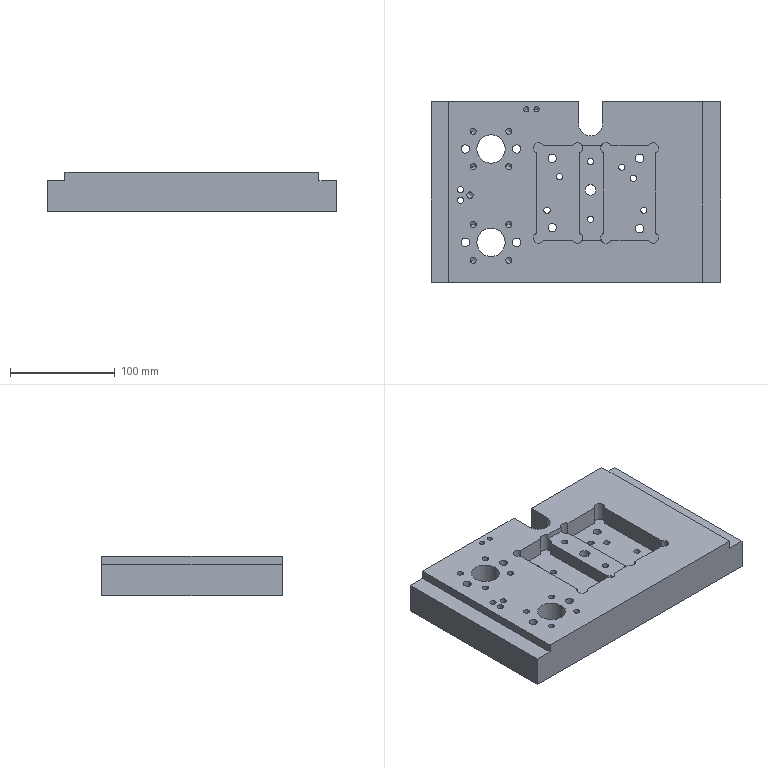Part | 1 solid | 119 faces | box 275.4 x 172 x 38 mm | volume 1497527 mm3 | cylinder 71 | plane 26 | cone 22 | commonest cylinder face diameters 6 x36 8 x16 10 x10 5 x4 27 x4 23 x1